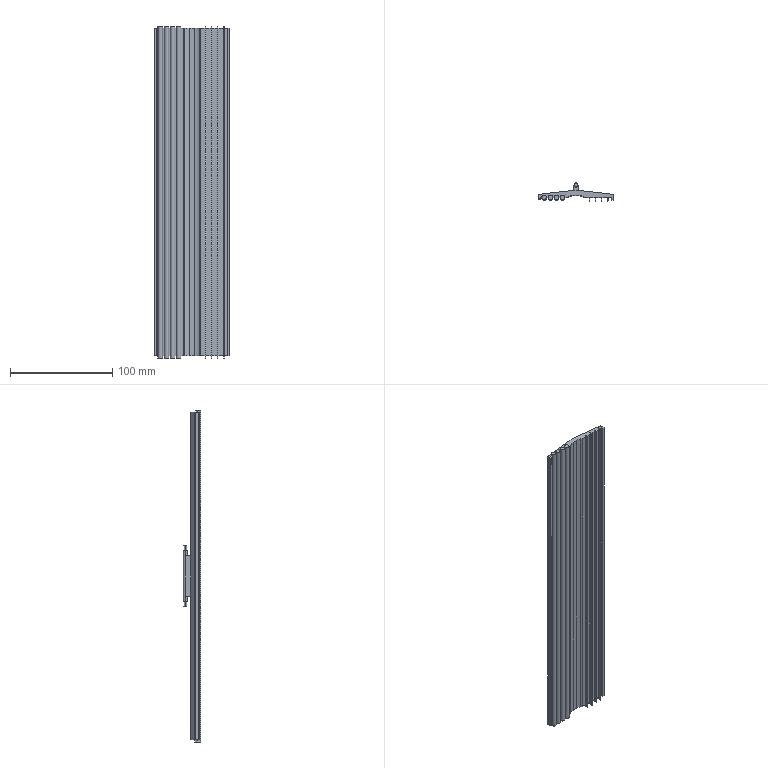Part | SolidWorks | features BaseBody 1 | 1 solid | 102 faces | box 73.253 x 17.318 x 324 mm | volume 124814 mm3 | plane 68 | cylinder 34 | commonest cylinder face diameters 4.5 x12 0.2 x8 2 x4 3 x4 4 x3 20 x2